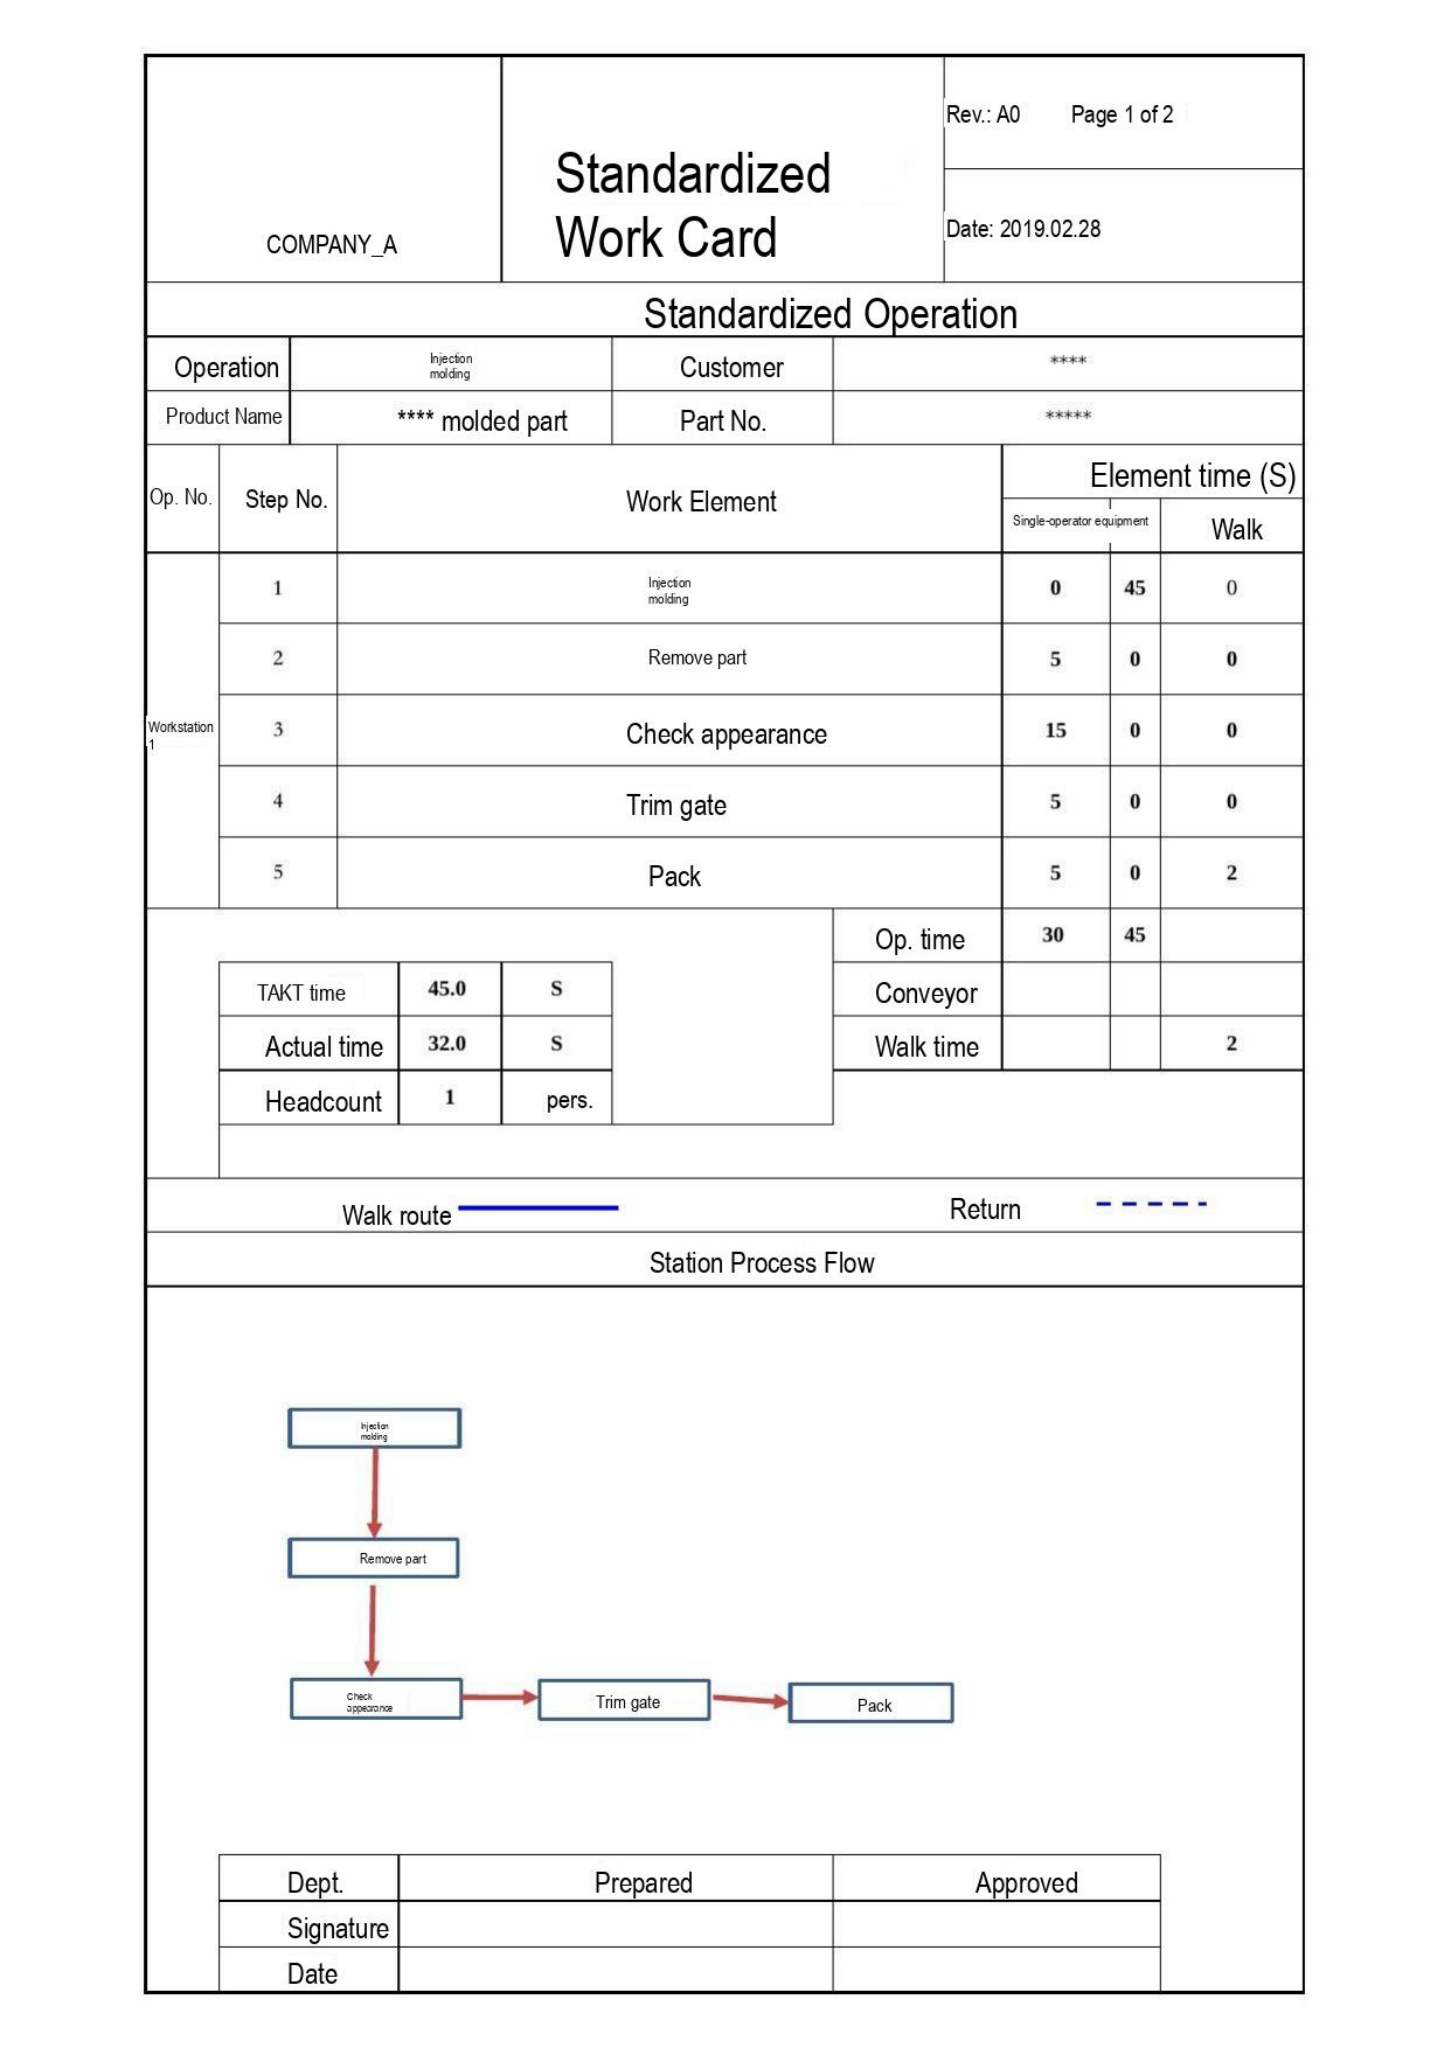| COMPANY_A | Standardized Work Card | Rev.: A0 Page 1 of 2 |
|---|---|---|
| | | Date: 2019.02.28 |

Standardized Operation

| Operation | Injection molding | Customer | **** |
|---|---|---|---|
| Product Name | **** molded part | Part No. | ***** |

| Op. No. | Step No. | Work Element | Element time (S) Single-operator | equipment | Walk |
|---|---|---|---|---|---|
| Workstation 1 | 1 | Injection molding | 0 | 45 | 0 |
| | 2 | Remove part | 5 | 0 | 0 |
| | 3 | Check appearance | 15 | 0 | 0 |
| | 4 | Trim gate | 5 | 0 | 0 |
| | 5 | Pack | 5 | 0 | 2 |
| | | Op. time | 30 | 45 | |
| | | Conveyor | | | |
| | | Walk time | | | 2 |

| TAKT time | 45.0 | S |
|---|---|---|
| Actual time | 32.0 | S |
| Headcount | 1 | pers. |

Walk route

Return

Station Process Flow

Injection molding

Remove part

Check appearance

Trim gate

Pack

| Dept. | Prepared | Approved |
|---|---|---|
| Signature | | |
| Date | | |
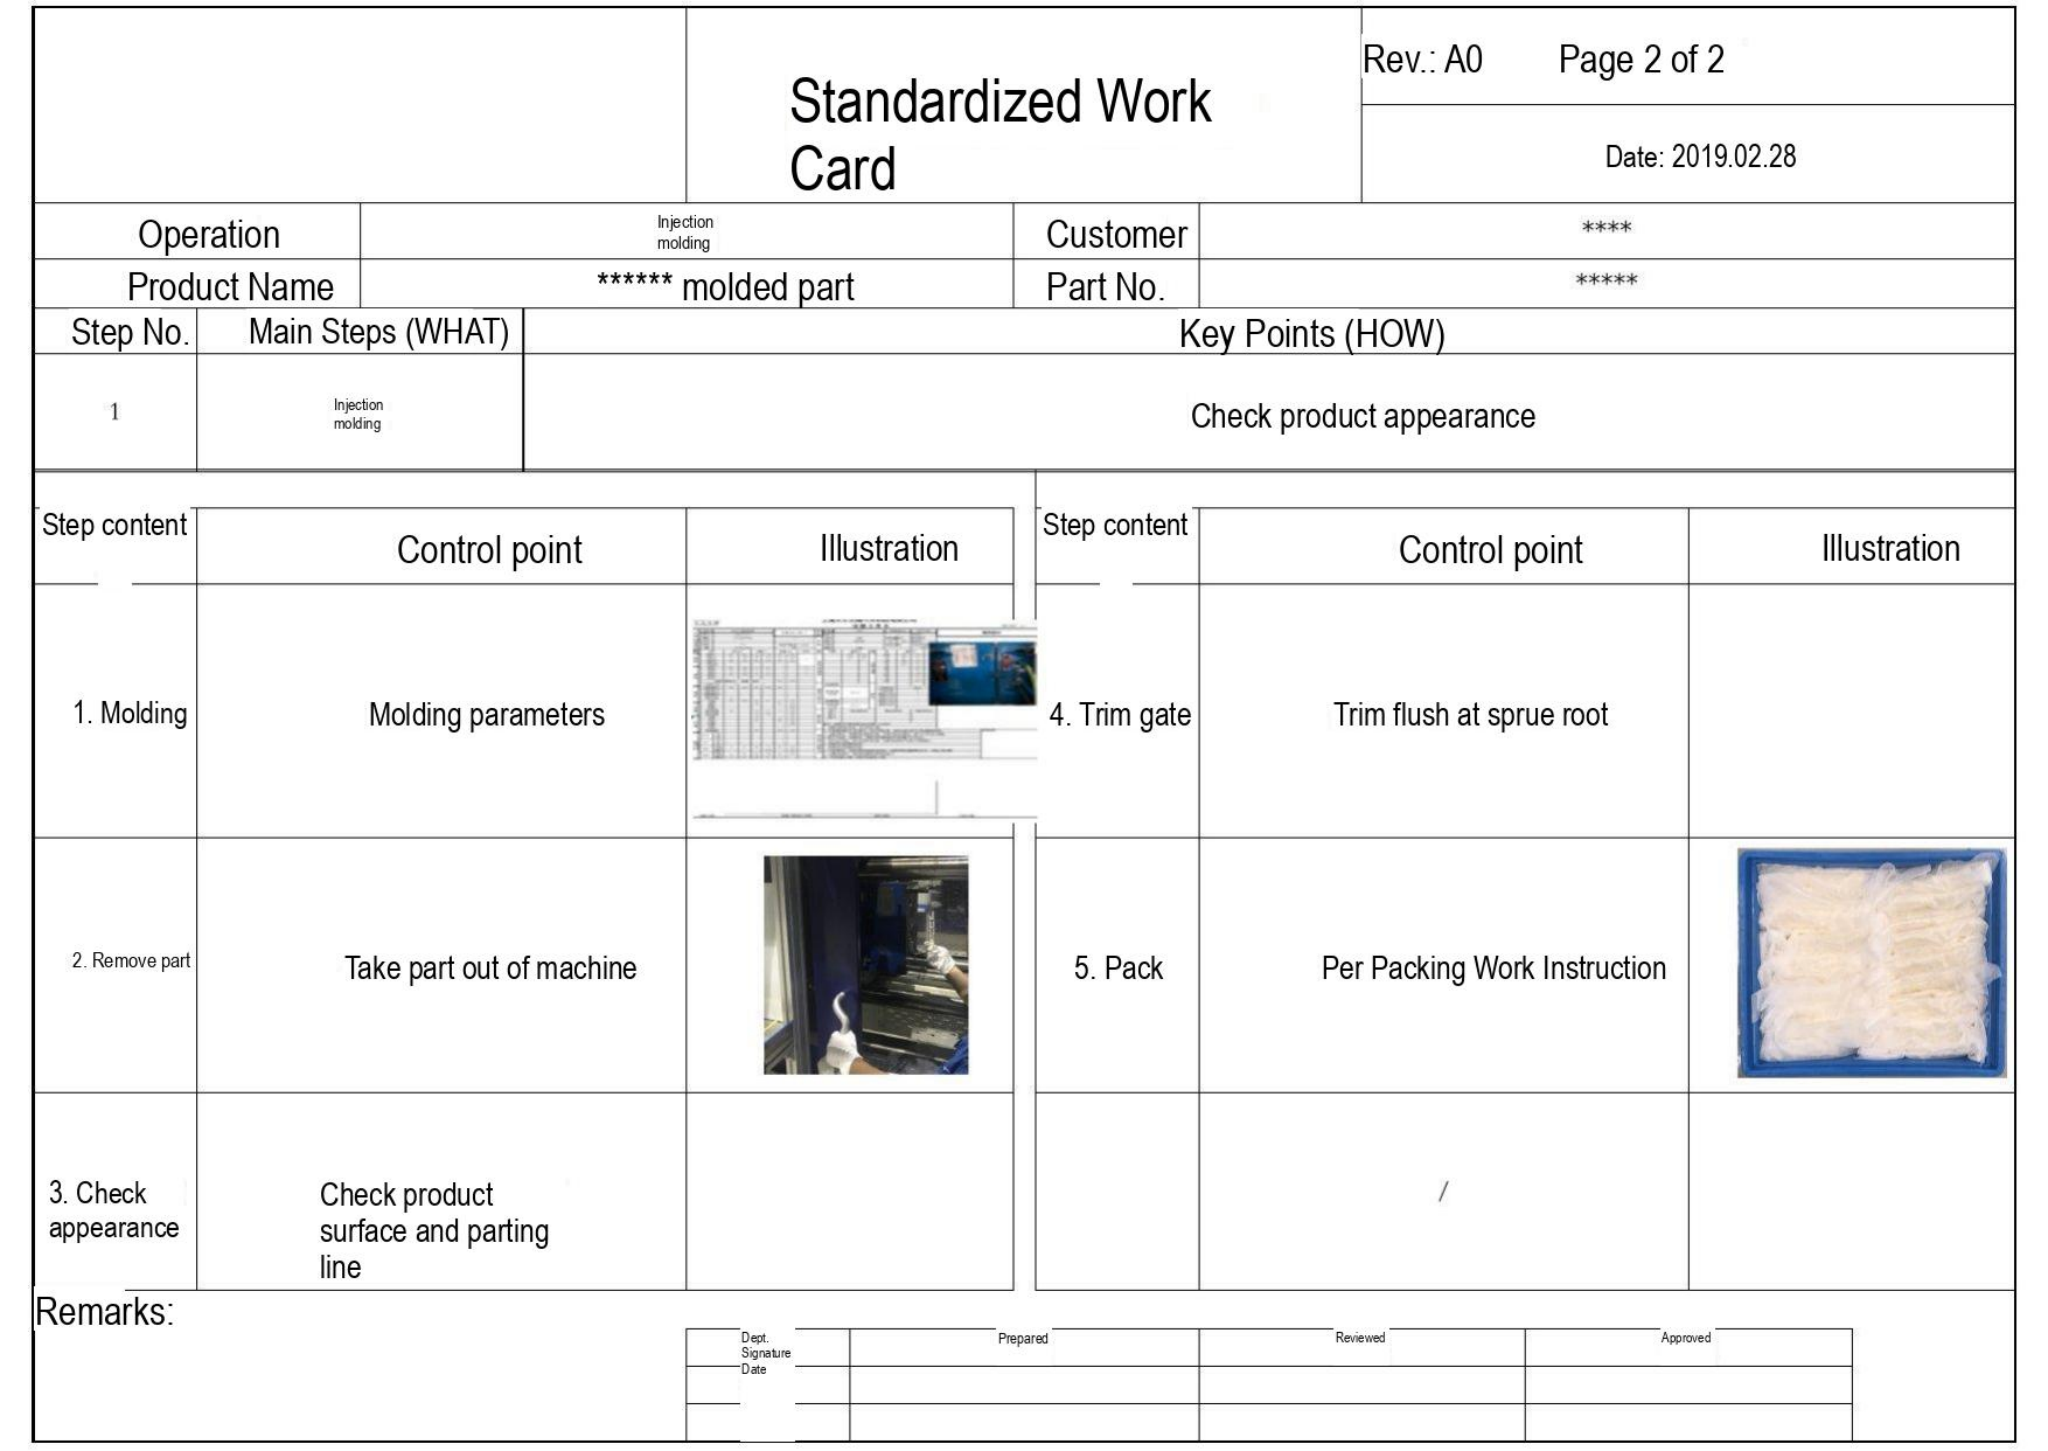Standardized Work Card

Rev.: A0 Page 2 of 2

Date: 2019.02.28

| Operation | Injection molding | Customer | **** |
|---|---|---|---|
| Product Name | ****** molded part | Part No. | ***** |

| Step No. | Main Steps (WHAT) | Key Points (HOW) |
|---|---|---|
| 1 | Injection molding | Check product appearance |

| Step content | Control point | Illustration | Step content | Control point | Illustration |
|---|---|---|---|---|---|
| 1. Molding | Molding parameters | | 4. Trim gate | Trim flush at sprue root | |
| 2. Remove part | Take part out of machine | | 5. Pack | Per Packing Work Instruction | |
| 3. Check appearance | Check product surface and parting line | | | / | |

Remarks:

| Dept. Signature Date | Prepared | Reviewed | Approved |
|---|---|---|---|
| | | | |
| | | | |